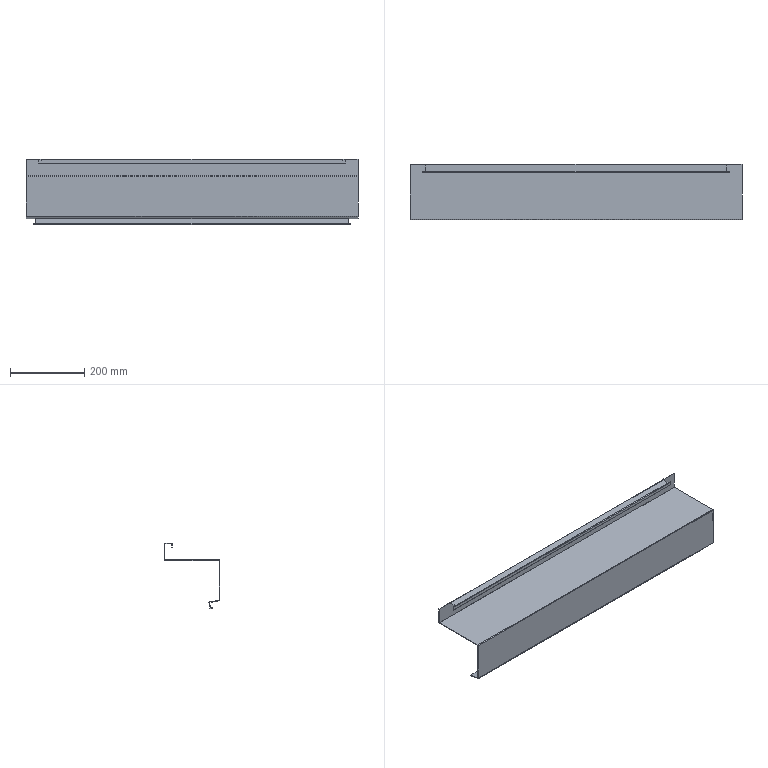Part | SolidWorks | features EdgeFlange 7, SMBaseFlange 3, FlatPattern 1, SheetMetal 1 | 1 solid | 94 faces | box 897 x 150.5 x 176.459 mm | volume 509426 mm3 | plane 80 | cylinder 14 | commonest cylinder face diameters 0.2 x7 3.2 x7